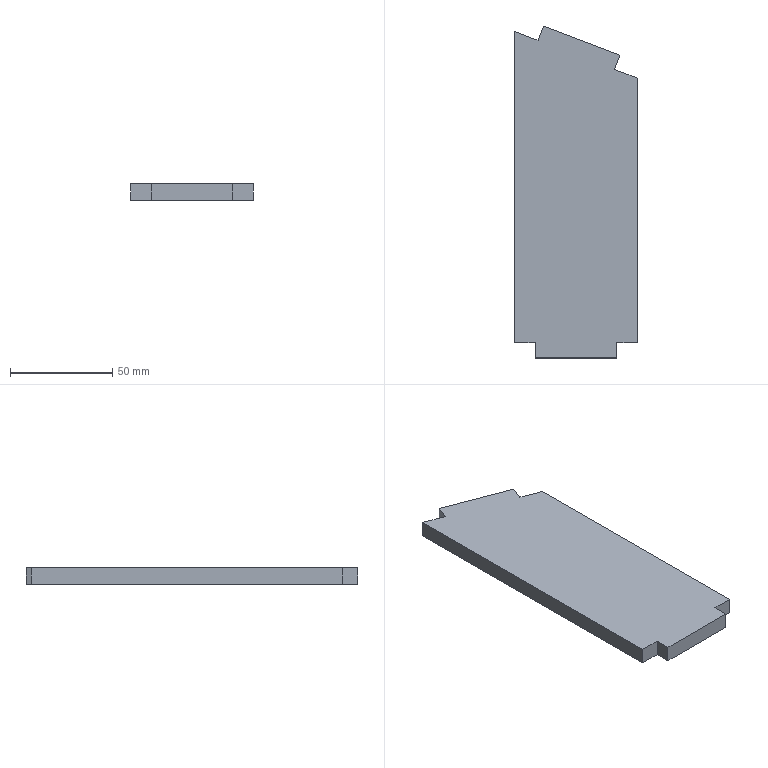Part | SolidWorks | features FlatPattern 1, SMBaseFlange 1, SheetMetal 1 | 1 solid | 14 faces | box 60 x 162.47 x 8 mm | volume 72422 mm3 | plane 14
STEP:
#1=CARTESIAN_POINT('',(-99.466,124.95,0.));
#2=VERTEX_POINT('',#1);
#3=CARTESIAN_POINT('',(-110.679,129.222,0.));
#4=VERTEX_POINT('',#3);
#5=CARTESIAN_POINT('',(-99.466,124.95,0.));
#6=DIRECTION('',(-0.9345,0.356,0.));
#7=VECTOR('',#6,1000.);
#8=LINE('',#5,#7);
#9=EDGE_CURVE('',#2,#4,#8,.T.);
#10=ORIENTED_EDGE('',*,*,#9,.T.);
#11=CARTESIAN_POINT('',(-110.679,129.222,8.));
#12=VERTEX_POINT('',#11);
#13=CARTESIAN_POINT('',(-110.679,129.222,8.));
#14=DIRECTION('',(0.,0.,-1.));
#15=VECTOR('',#14,1000.);
#16=LINE('',#13,#15);
#17=EDGE_CURVE('',#12,#4,#16,.T.);
#18=ORIENTED_EDGE('',*,*,#17,.F.);
#19=CARTESIAN_POINT('',(-99.466,124.95,8.));
#20=VERTEX_POINT('',#19);
#21=CARTESIAN_POINT('',(-99.466,124.95,8.));
#22=DIRECTION('',(-0.9345,0.356,0.));
#23=VECTOR('',#22,1000.);
#24=LINE('',#21,#23);
#25=EDGE_CURVE('',#20,#12,#24,.T.);
#26=ORIENTED_EDGE('',*,*,#25,.F.);
#27=CARTESIAN_POINT('',(-99.466,124.95,8.));
#28=DIRECTION('',(0.,0.,-1.));
#29=VECTOR('',#28,1000.);
#30=LINE('',#27,#29);
#31=EDGE_CURVE('',#20,#2,#30,.T.);
#32=ORIENTED_EDGE('',*,*,#31,.T.);
#33=EDGE_LOOP('',(#10,#18,#26,#32));
#34=FACE_OUTER_BOUND('',#33,.T.);
#35=CARTESIAN_POINT('',(-99.466,124.95,8.));
#36=DIRECTION('',(-0.356,-0.9345,0.));
#37=DIRECTION('',(0.9345,-0.356,0.));
#38=AXIS2_PLACEMENT_3D('',#35,#36,#37);
#39=PLANE('',#38);
#40=ADVANCED_FACE('',(#34),#39,.F.);
#41=CARTESIAN_POINT('',(-108.009,136.23,0.));
#42=VERTEX_POINT('',#41);
#43=CARTESIAN_POINT('',(-110.679,129.222,0.));
#44=DIRECTION('',(0.356,0.9345,0.));
#45=VECTOR('',#44,1000.);
#46=LINE('',#43,#45);
#47=EDGE_CURVE('',#4,#42,#46,.T.);
#48=ORIENTED_EDGE('',*,*,#47,.T.);
#49=CARTESIAN_POINT('',(-108.009,136.23,8.));
#50=VERTEX_POINT('',#49);
#51=CARTESIAN_POINT('',(-108.009,136.23,8.));
#52=DIRECTION('',(0.,0.,-1.));
#53=VECTOR('',#52,1000.);
#54=LINE('',#51,#53);
#55=EDGE_CURVE('',#50,#42,#54,.T.);
#56=ORIENTED_EDGE('',*,*,#55,.F.);
#57=CARTESIAN_POINT('',(-110.679,129.222,8.));
#58=DIRECTION('',(0.356,0.9345,0.));
#59=VECTOR('',#58,1000.);
#60=LINE('',#57,#59);
#61=EDGE_CURVE('',#12,#50,#60,.T.);
#62=ORIENTED_EDGE('',*,*,#61,.F.);
#63=ORIENTED_EDGE('',*,*,#17,.T.);
#64=EDGE_LOOP('',(#48,#56,#62,#63));
#65=FACE_OUTER_BOUND('',#64,.T.);
#66=CARTESIAN_POINT('',(-110.679,129.222,8.));
#67=DIRECTION('',(-0.9345,0.356,0.));
#68=DIRECTION('',(-0.356,-0.9345,0.));
#69=AXIS2_PLACEMENT_3D('',#66,#67,#68);
#70=PLANE('',#69);
#71=ADVANCED_FACE('',(#65),#70,.F.);
#72=CARTESIAN_POINT('',(-145.389,150.47,0.));
#73=VERTEX_POINT('',#72);
#74=CARTESIAN_POINT('',(-108.009,136.23,0.));
#75=DIRECTION('',(-0.9345,0.356,0.));
#76=VECTOR('',#75,1000.);
#77=LINE('',#74,#76);
#78=EDGE_CURVE('',#42,#73,#77,.T.);
#79=ORIENTED_EDGE('',*,*,#78,.T.);
#80=CARTESIAN_POINT('',(-145.389,150.47,8.));
#81=VERTEX_POINT('',#80);
#82=CARTESIAN_POINT('',(-145.389,150.47,8.));
#83=DIRECTION('',(0.,0.,-1.));
#84=VECTOR('',#83,1000.);
#85=LINE('',#82,#84);
#86=EDGE_CURVE('',#81,#73,#85,.T.);
#87=ORIENTED_EDGE('',*,*,#86,.F.);
#88=CARTESIAN_POINT('',(-108.009,136.23,8.));
#89=DIRECTION('',(-0.9345,0.356,0.));
#90=VECTOR('',#89,1000.);
#91=LINE('',#88,#90);
#92=EDGE_CURVE('',#50,#81,#91,.T.);
#93=ORIENTED_EDGE('',*,*,#92,.F.);
#94=ORIENTED_EDGE('',*,*,#55,.T.);
#95=EDGE_LOOP('',(#79,#87,#93,#94));
#96=FACE_OUTER_BOUND('',#95,.T.);
#97=CARTESIAN_POINT('',(-108.009,136.23,8.));
#98=DIRECTION('',(-0.356,-0.9345,0.));
#99=DIRECTION('',(0.9345,-0.356,0.));
#100=AXIS2_PLACEMENT_3D('',#97,#98,#99);
#101=PLANE('',#100);
#102=ADVANCED_FACE('',(#96),#101,.F.);
#103=CARTESIAN_POINT('',(-148.059,143.462,0.));
#104=VERTEX_POINT('',#103);
#105=CARTESIAN_POINT('',(-145.389,150.47,0.));
#106=DIRECTION('',(-0.356,-0.9345,0.));
#107=VECTOR('',#106,1000.);
#108=LINE('',#105,#107);
#109=EDGE_CURVE('',#73,#104,#108,.T.);
#110=ORIENTED_EDGE('',*,*,#109,.T.);
#111=CARTESIAN_POINT('',(-148.059,143.462,8.));
#112=VERTEX_POINT('',#111);
#113=CARTESIAN_POINT('',(-148.059,143.462,8.));
#114=DIRECTION('',(0.,0.,-1.));
#115=VECTOR('',#114,1000.);
#116=LINE('',#113,#115);
#117=EDGE_CURVE('',#112,#104,#116,.T.);
#118=ORIENTED_EDGE('',*,*,#117,.F.);
#119=CARTESIAN_POINT('',(-145.389,150.47,8.));
#120=DIRECTION('',(-0.356,-0.9345,0.));
#121=VECTOR('',#120,1000.);
#122=LINE('',#119,#121);
#123=EDGE_CURVE('',#81,#112,#122,.T.);
#124=ORIENTED_EDGE('',*,*,#123,.F.);
#125=ORIENTED_EDGE('',*,*,#86,.T.);
#126=EDGE_LOOP('',(#110,#118,#124,#125));
#127=FACE_OUTER_BOUND('',#126,.T.);
#128=CARTESIAN_POINT('',(-145.389,150.47,8.));
#129=DIRECTION('',(0.9345,-0.356,0.));
#130=DIRECTION('',(0.356,0.9345,0.));
#131=AXIS2_PLACEMENT_3D('',#128,#129,#130);
#132=PLANE('',#131);
#133=ADVANCED_FACE('',(#127),#132,.F.);
#134=CARTESIAN_POINT('',(-159.466,147.807,0.));
#135=VERTEX_POINT('',#134);
#136=CARTESIAN_POINT('',(-148.059,143.462,0.));
#137=DIRECTION('',(-0.9345,0.356,0.));
#138=VECTOR('',#137,1000.);
#139=LINE('',#136,#138);
#140=EDGE_CURVE('',#104,#135,#139,.T.);
#141=ORIENTED_EDGE('',*,*,#140,.T.);
#142=CARTESIAN_POINT('',(-159.466,147.807,8.));
#143=VERTEX_POINT('',#142);
#144=CARTESIAN_POINT('',(-159.466,147.807,8.));
#145=DIRECTION('',(0.,0.,-1.));
#146=VECTOR('',#145,1000.);
#147=LINE('',#144,#146);
#148=EDGE_CURVE('',#143,#135,#147,.T.);
#149=ORIENTED_EDGE('',*,*,#148,.F.);
#150=CARTESIAN_POINT('',(-148.059,143.462,8.));
#151=DIRECTION('',(-0.9345,0.356,0.));
#152=VECTOR('',#151,1000.);
#153=LINE('',#150,#152);
#154=EDGE_CURVE('',#112,#143,#153,.T.);
#155=ORIENTED_EDGE('',*,*,#154,.F.);
#156=ORIENTED_EDGE('',*,*,#117,.T.);
#157=EDGE_LOOP('',(#141,#149,#155,#156));
#158=FACE_OUTER_BOUND('',#157,.T.);
#159=CARTESIAN_POINT('',(-148.059,143.462,8.));
#160=DIRECTION('',(-0.356,-0.9345,0.));
#161=DIRECTION('',(0.9345,-0.356,0.));
#162=AXIS2_PLACEMENT_3D('',#159,#160,#161);
#163=PLANE('',#162);
#164=ADVANCED_FACE('',(#158),#163,.F.);
#165=CARTESIAN_POINT('',(-159.466,-4.5,0.));
#166=VERTEX_POINT('',#165);
#167=CARTESIAN_POINT('',(-159.466,147.807,0.));
#168=DIRECTION('',(0.,-1.,0.));
#169=VECTOR('',#168,1000.);
#170=LINE('',#167,#169);
#171=EDGE_CURVE('',#135,#166,#170,.T.);
#172=ORIENTED_EDGE('',*,*,#171,.T.);
#173=CARTESIAN_POINT('',(-159.466,-4.5,8.));
#174=VERTEX_POINT('',#173);
#175=CARTESIAN_POINT('',(-159.466,-4.5,8.));
#176=DIRECTION('',(0.,0.,-1.));
#177=VECTOR('',#176,1000.);
#178=LINE('',#175,#177);
#179=EDGE_CURVE('',#174,#166,#178,.T.);
#180=ORIENTED_EDGE('',*,*,#179,.F.);
#181=CARTESIAN_POINT('',(-159.466,147.807,8.));
#182=DIRECTION('',(0.,-1.,0.));
#183=VECTOR('',#182,1000.);
#184=LINE('',#181,#183);
#185=EDGE_CURVE('',#143,#174,#184,.T.);
#186=ORIENTED_EDGE('',*,*,#185,.F.);
#187=ORIENTED_EDGE('',*,*,#148,.T.);
#188=EDGE_LOOP('',(#172,#180,#186,#187));
#189=FACE_OUTER_BOUND('',#188,.T.);
#190=CARTESIAN_POINT('',(-159.466,147.807,8.));
#191=DIRECTION('',(1.,0.,0.));
#192=DIRECTION('',(0.,1.,0.));
#193=AXIS2_PLACEMENT_3D('',#190,#191,#192);
#194=PLANE('',#193);
#195=ADVANCED_FACE('',(#189),#194,.F.);
#196=CARTESIAN_POINT('',(-149.466,-4.5,0.));
#197=VERTEX_POINT('',#196);
#198=CARTESIAN_POINT('',(-149.466,-4.5,0.));
#199=DIRECTION('',(1.,0.,0.));
#200=VECTOR('',#199,1000.);
#201=LINE('',#198,#200);
#202=EDGE_CURVE('',#166,#197,#201,.T.);
#203=ORIENTED_EDGE('',*,*,#202,.T.);
#204=CARTESIAN_POINT('',(-149.466,-4.5,8.));
#205=VERTEX_POINT('',#204);
#206=CARTESIAN_POINT('',(-149.466,-4.5,8.));
#207=DIRECTION('',(0.,0.,-1.));
#208=VECTOR('',#207,1000.);
#209=LINE('',#206,#208);
#210=EDGE_CURVE('',#205,#197,#209,.T.);
#211=ORIENTED_EDGE('',*,*,#210,.F.);
#212=CARTESIAN_POINT('',(-149.466,-4.5,8.));
#213=DIRECTION('',(1.,0.,0.));
#214=VECTOR('',#213,1000.);
#215=LINE('',#212,#214);
#216=EDGE_CURVE('',#174,#205,#215,.T.);
#217=ORIENTED_EDGE('',*,*,#216,.F.);
#218=ORIENTED_EDGE('',*,*,#179,.T.);
#219=EDGE_LOOP('',(#203,#211,#217,#218));
#220=FACE_OUTER_BOUND('',#219,.T.);
#221=CARTESIAN_POINT('',(-149.466,-4.5,8.));
#222=DIRECTION('',(0.,1.,0.));
#223=DIRECTION('',(-1.,0.,0.));
#224=AXIS2_PLACEMENT_3D('',#221,#222,#223);
#225=PLANE('',#224);
#226=ADVANCED_FACE('',(#220),#225,.F.);
#227=CARTESIAN_POINT('',(-149.466,-12.,0.));
#228=VERTEX_POINT('',#227);
#229=CARTESIAN_POINT('',(-149.466,-4.5,0.));
#230=DIRECTION('',(0.,-1.,0.));
#231=VECTOR('',#230,1000.);
#232=LINE('',#229,#231);
#233=EDGE_CURVE('',#197,#228,#232,.T.);
#234=ORIENTED_EDGE('',*,*,#233,.T.);
#235=CARTESIAN_POINT('',(-149.466,-12.,8.));
#236=VERTEX_POINT('',#235);
#237=CARTESIAN_POINT('',(-149.466,-12.,8.));
#238=DIRECTION('',(0.,0.,-1.));
#239=VECTOR('',#238,1000.);
#240=LINE('',#237,#239);
#241=EDGE_CURVE('',#236,#228,#240,.T.);
#242=ORIENTED_EDGE('',*,*,#241,.F.);
#243=CARTESIAN_POINT('',(-149.466,-4.5,8.));
#244=DIRECTION('',(0.,-1.,0.));
#245=VECTOR('',#244,1000.);
#246=LINE('',#243,#245);
#247=EDGE_CURVE('',#205,#236,#246,.T.);
#248=ORIENTED_EDGE('',*,*,#247,.F.);
#249=ORIENTED_EDGE('',*,*,#210,.T.);
#250=EDGE_LOOP('',(#234,#242,#248,#249));
#251=FACE_OUTER_BOUND('',#250,.T.);
#252=CARTESIAN_POINT('',(-149.466,-4.5,8.));
#253=DIRECTION('',(1.,0.,0.));
#254=DIRECTION('',(0.,0.,-1.));
#255=AXIS2_PLACEMENT_3D('',#252,#253,#254);
#256=PLANE('',#255);
#257=ADVANCED_FACE('',(#251),#256,.F.);
#258=CARTESIAN_POINT('',(-109.466,-12.,0.));
#259=VERTEX_POINT('',#258);
#260=CARTESIAN_POINT('',(-149.466,-12.,0.));
#261=DIRECTION('',(1.,0.,0.));
#262=VECTOR('',#261,1000.);
#263=LINE('',#260,#262);
#264=EDGE_CURVE('',#228,#259,#263,.T.);
#265=ORIENTED_EDGE('',*,*,#264,.T.);
#266=CARTESIAN_POINT('',(-109.466,-12.,8.));
#267=VERTEX_POINT('',#266);
#268=CARTESIAN_POINT('',(-109.466,-12.,8.));
#269=DIRECTION('',(0.,0.,-1.));
#270=VECTOR('',#269,1000.);
#271=LINE('',#268,#270);
#272=EDGE_CURVE('',#267,#259,#271,.T.);
#273=ORIENTED_EDGE('',*,*,#272,.F.);
#274=CARTESIAN_POINT('',(-149.466,-12.,8.));
#275=DIRECTION('',(1.,0.,0.));
#276=VECTOR('',#275,1000.);
#277=LINE('',#274,#276);
#278=EDGE_CURVE('',#236,#267,#277,.T.);
#279=ORIENTED_EDGE('',*,*,#278,.F.);
#280=ORIENTED_EDGE('',*,*,#241,.T.);
#281=EDGE_LOOP('',(#265,#273,#279,#280));
#282=FACE_OUTER_BOUND('',#281,.T.);
#283=CARTESIAN_POINT('',(-149.466,-12.,8.));
#284=DIRECTION('',(0.,1.,0.));
#285=DIRECTION('',(0.,0.,1.));
#286=AXIS2_PLACEMENT_3D('',#283,#284,#285);
#287=PLANE('',#286);
#288=ADVANCED_FACE('',(#282),#287,.F.);
#289=CARTESIAN_POINT('',(-109.466,-4.5,0.));
#290=VERTEX_POINT('',#289);
#291=CARTESIAN_POINT('',(-109.466,-12.,0.));
#292=DIRECTION('',(0.,1.,0.));
#293=VECTOR('',#292,1000.);
#294=LINE('',#291,#293);
#295=EDGE_CURVE('',#259,#290,#294,.T.);
#296=ORIENTED_EDGE('',*,*,#295,.T.);
#297=CARTESIAN_POINT('',(-109.466,-4.5,8.));
#298=VERTEX_POINT('',#297);
#299=CARTESIAN_POINT('',(-109.466,-4.5,8.));
#300=DIRECTION('',(0.,0.,-1.));
#301=VECTOR('',#300,1000.);
#302=LINE('',#299,#301);
#303=EDGE_CURVE('',#298,#290,#302,.T.);
#304=ORIENTED_EDGE('',*,*,#303,.F.);
#305=CARTESIAN_POINT('',(-109.466,-12.,8.));
#306=DIRECTION('',(0.,1.,0.));
#307=VECTOR('',#306,1000.);
#308=LINE('',#305,#307);
#309=EDGE_CURVE('',#267,#298,#308,.T.);
#310=ORIENTED_EDGE('',*,*,#309,.F.);
#311=ORIENTED_EDGE('',*,*,#272,.T.);
#312=EDGE_LOOP('',(#296,#304,#310,#311));
#313=FACE_OUTER_BOUND('',#312,.T.);
#314=CARTESIAN_POINT('',(-109.466,-12.,8.));
#315=DIRECTION('',(-1.,0.,0.));
#316=DIRECTION('',(0.,0.,1.));
#317=AXIS2_PLACEMENT_3D('',#314,#315,#316);
#318=PLANE('',#317);
#319=ADVANCED_FACE('',(#313),#318,.F.);
#320=CARTESIAN_POINT('',(-99.466,-4.5,0.));
#321=VERTEX_POINT('',#320);
#322=CARTESIAN_POINT('',(-99.466,-4.5,0.));
#323=DIRECTION('',(1.,0.,0.));
#324=VECTOR('',#323,1000.);
#325=LINE('',#322,#324);
#326=EDGE_CURVE('',#290,#321,#325,.T.);
#327=ORIENTED_EDGE('',*,*,#326,.T.);
#328=CARTESIAN_POINT('',(-99.466,-4.5,8.));
#329=VERTEX_POINT('',#328);
#330=CARTESIAN_POINT('',(-99.466,-4.5,8.));
#331=DIRECTION('',(0.,0.,-1.));
#332=VECTOR('',#331,1000.);
#333=LINE('',#330,#332);
#334=EDGE_CURVE('',#329,#321,#333,.T.);
#335=ORIENTED_EDGE('',*,*,#334,.F.);
#336=CARTESIAN_POINT('',(-99.466,-4.5,8.));
#337=DIRECTION('',(1.,0.,0.));
#338=VECTOR('',#337,1000.);
#339=LINE('',#336,#338);
#340=EDGE_CURVE('',#298,#329,#339,.T.);
#341=ORIENTED_EDGE('',*,*,#340,.F.);
#342=ORIENTED_EDGE('',*,*,#303,.T.);
#343=EDGE_LOOP('',(#327,#335,#341,#342));
#344=FACE_OUTER_BOUND('',#343,.T.);
#345=CARTESIAN_POINT('',(-99.466,-4.5,8.));
#346=DIRECTION('',(0.,1.,0.));
#347=DIRECTION('',(0.,0.,1.));
#348=AXIS2_PLACEMENT_3D('',#345,#346,#347);
#349=PLANE('',#348);
#350=ADVANCED_FACE('',(#344),#349,.F.);
#351=CARTESIAN_POINT('',(-99.466,124.95,0.));
#352=DIRECTION('',(0.,1.,0.));
#353=VECTOR('',#352,1000.);
#354=LINE('',#351,#353);
#355=EDGE_CURVE('',#321,#2,#354,.T.);
#356=ORIENTED_EDGE('',*,*,#355,.T.);
#357=ORIENTED_EDGE('',*,*,#31,.F.);
#358=CARTESIAN_POINT('',(-99.466,124.95,8.));
#359=DIRECTION('',(0.,1.,0.));
#360=VECTOR('',#359,1000.);
#361=LINE('',#358,#360);
#362=EDGE_CURVE('',#329,#20,#361,.T.);
#363=ORIENTED_EDGE('',*,*,#362,.F.);
#364=ORIENTED_EDGE('',*,*,#334,.T.);
#365=EDGE_LOOP('',(#356,#357,#363,#364));
#366=FACE_OUTER_BOUND('',#365,.T.);
#367=CARTESIAN_POINT('',(-99.466,124.95,8.));
#368=DIRECTION('',(-1.,0.,0.));
#369=DIRECTION('',(0.,-1.,0.));
#370=AXIS2_PLACEMENT_3D('',#367,#368,#369);
#371=PLANE('',#370);
#372=ADVANCED_FACE('',(#366),#371,.F.);
#373=ORIENTED_EDGE('',*,*,#25,.T.);
#374=ORIENTED_EDGE('',*,*,#61,.T.);
#375=ORIENTED_EDGE('',*,*,#92,.T.);
#376=ORIENTED_EDGE('',*,*,#123,.T.);
#377=ORIENTED_EDGE('',*,*,#154,.T.);
#378=ORIENTED_EDGE('',*,*,#185,.T.);
#379=ORIENTED_EDGE('',*,*,#216,.T.);
#380=ORIENTED_EDGE('',*,*,#247,.T.);
#381=ORIENTED_EDGE('',*,*,#278,.T.);
#382=ORIENTED_EDGE('',*,*,#309,.T.);
#383=ORIENTED_EDGE('',*,*,#340,.T.);
#384=ORIENTED_EDGE('',*,*,#362,.T.);
#385=EDGE_LOOP('',(#373,#374,#375,#376,#377,#378,#379,#380,#381,#382,#383,#384));
#386=FACE_OUTER_BOUND('',#385,.T.);
#387=CARTESIAN_POINT('',(0.,0.,8.));
#388=DIRECTION('',(0.,0.,-1.));
#389=DIRECTION('',(-1.,0.,0.));
#390=AXIS2_PLACEMENT_3D('',#387,#388,#389);
#391=PLANE('',#390);
#392=ADVANCED_FACE('',(#386),#391,.F.);
#393=ORIENTED_EDGE('',*,*,#9,.F.);
#394=ORIENTED_EDGE('',*,*,#355,.F.);
#395=ORIENTED_EDGE('',*,*,#326,.F.);
#396=ORIENTED_EDGE('',*,*,#295,.F.);
#397=ORIENTED_EDGE('',*,*,#264,.F.);
#398=ORIENTED_EDGE('',*,*,#233,.F.);
#399=ORIENTED_EDGE('',*,*,#202,.F.);
#400=ORIENTED_EDGE('',*,*,#171,.F.);
#401=ORIENTED_EDGE('',*,*,#140,.F.);
#402=ORIENTED_EDGE('',*,*,#109,.F.);
#403=ORIENTED_EDGE('',*,*,#78,.F.);
#404=ORIENTED_EDGE('',*,*,#47,.F.);
#405=EDGE_LOOP('',(#393,#394,#395,#396,#397,#398,#399,#400,#401,#402,#403,#404));
#406=FACE_OUTER_BOUND('',#405,.T.);
#407=CARTESIAN_POINT('',(0.,0.,0.));
#408=DIRECTION('',(0.,0.,-1.));
#409=DIRECTION('',(-1.,0.,0.));
#410=AXIS2_PLACEMENT_3D('',#407,#408,#409);
#411=PLANE('',#410);
#412=ADVANCED_FACE('',(#406),#411,.T.);
#413=CLOSED_SHELL('',(#40,#71,#102,#133,#164,#195,#226,#257,#288,#319,#350,#372,#392,#412));
#414=MANIFOLD_SOLID_BREP('',#413);
#415=CARTESIAN_POINT('',(0.,0.,0.));
#416=DIRECTION('',(0.,0.,1.));
#417=DIRECTION('',(1.,0.,0.));
#418=AXIS2_PLACEMENT_3D('',#415,#416,#417);
#419=(LENGTH_UNIT()NAMED_UNIT(*)SI_UNIT(.MILLI.,.METRE.));
#420=UNCERTAINTY_MEASURE_WITH_UNIT(LENGTH_MEASURE(0.00001),#419,'','');
#421=(NAMED_UNIT(*)PLANE_ANGLE_UNIT()SI_UNIT($,.RADIAN.));
#422=(NAMED_UNIT(*)SI_UNIT($,.STERADIAN.)SOLID_ANGLE_UNIT());
#423=(GEOMETRIC_REPRESENTATION_CONTEXT(3)GLOBAL_UNCERTAINTY_ASSIGNED_CONTEXT((#420))GLOBAL_UNIT_ASSIGNED_CONTEXT((#419,#421,#422))REPRESENTATION_CONTEXT('',''));
#424=ADVANCED_BREP_SHAPE_REPRESENTATION('',(#414,#418),#423);